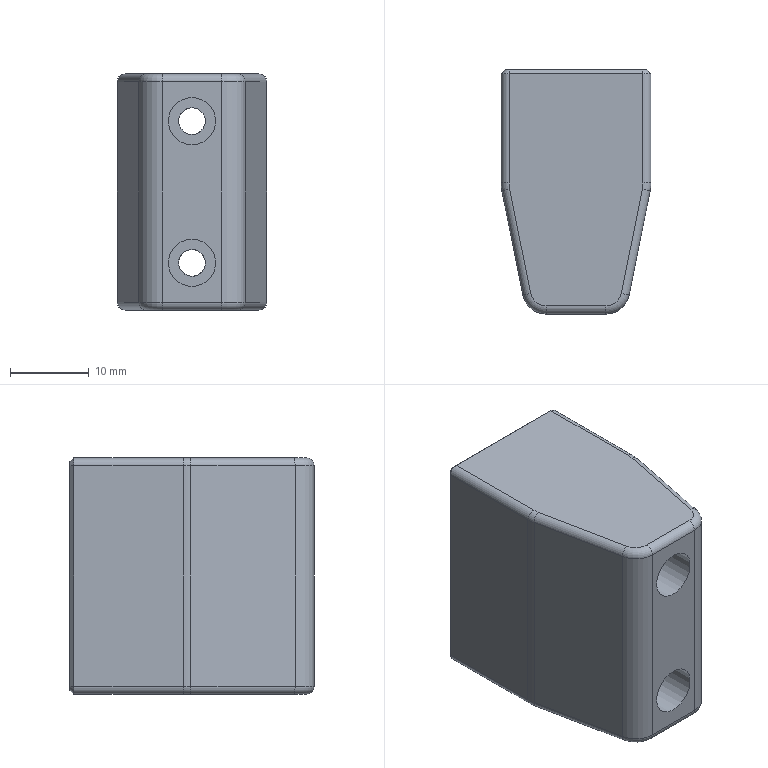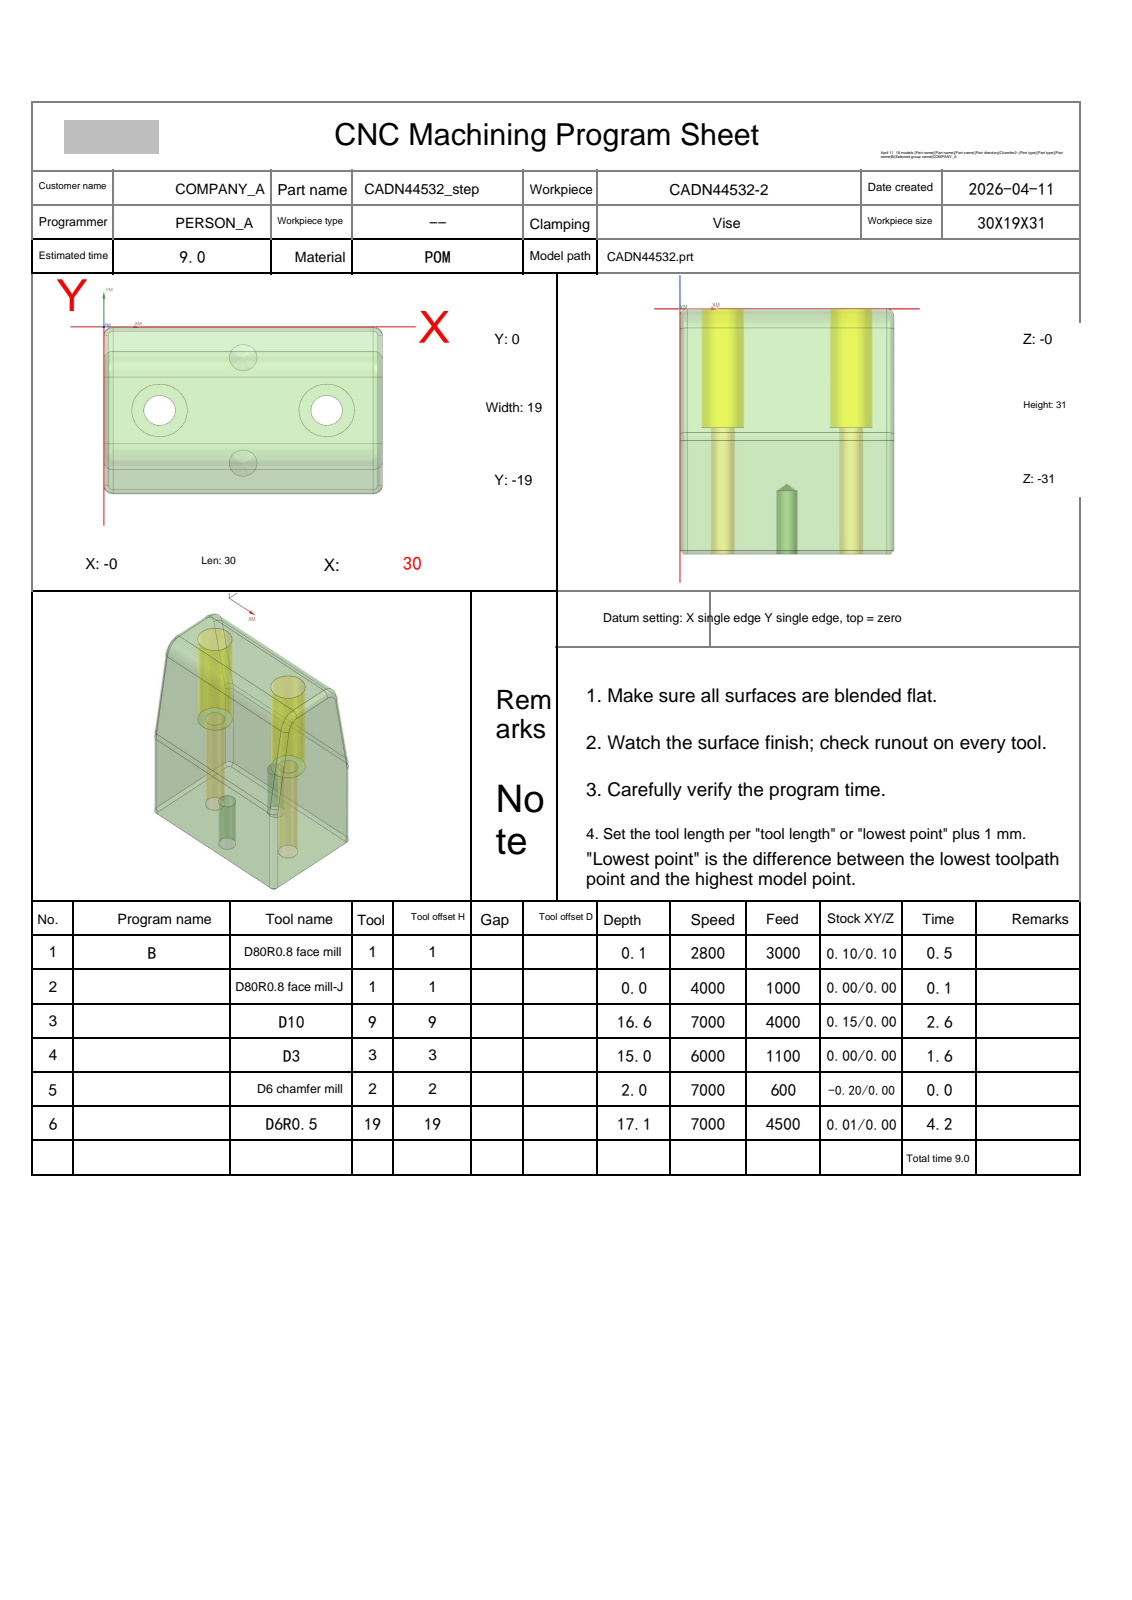NC program | NX | posted by the shop | part box 19 x 31 x 30 mm
Lines 2365 to 3536 of 6576:
N6 T19 M06
(D6R0.5  D=6. R=0.5 H=19 ce=0.01 di=0.00)
G00 G90 G54 X-2.86 Y-7.974 M03 S7000
G43 H19 Z14.8
M08
Z.492
G01 Z-.008 F4500.
G03 X-1.66 Y-6.816 I0.0 J1.2
G01 X-1.618 Y-5.615
G02 X1. Y-2.966 I2.746 J-.096
G01 X29.
G02 X31.633 Y-5.668 I-.14 J-2.77
G01 X31.66 Y-6.816
X31.702 Z-.012
X31.737 Z-.017
X31.725 Y-5.724
G03 X29. Y-2.849 I-2.912 J-.031
G01 X.999
G03 X-1.489 Y-4.634 I0.0 J-2.627
X-1.763 Y-6.296 I4.913 J-1.662
X-1.737 Y-6.816 I5.186 J0.0
G01 X-1.774 Z-.023
X-1.807 Z-.03
G02 X-1.83 Y-6.298 I5.824 J.518
X-1.667 Y-4.927 I5.847 J0.0
X1. Y-2.741 I2.779 J-.671
G01 X29.
G02 X31.795 Y-5.662 I-.16 J-2.951
G01 X31.807 Y-6.816
X31.843 Z-.037
X31.876 Z-.045
X31.863 Y-5.621
G03 X29. Y-2.635 I-3.023 J-.033
G01 X1.
G03 X-1.867 Y-5.661 I.164 J-3.027
G01 Y-5.666
X-1.865 Y-6.558
X-1.876 Y-6.816
X-1.91 Z-.054
X-1.942 Z-.063
G02 X-1.957 Y-6.31 I8.273 J.506
X-1.879 Y-5.173 I8.288 J0.0
X1. Y-2.532 I3.015 J-.397
G01 X29.
G02 X31.879 Y-5.173 I-.136 J-3.038
X31.957 Y-6.31 I-8.21 J-1.137
X31.942 Y-6.816 I-8.288 J0.0
G01 X31.975 Z-.074
X32.006 Z-.085
G03 X32.011 Y-6.458 I-13.525 J.358
X31.958 Y-5.264 I-13.53 J0.0
X29. Y-2.431 I-3.098 J-.275
G01 X1.
G03 X-1.958 Y-5.264 I.14 J-3.107
X-2.011 Y-6.458 I13.477 J-1.194
X-2.006 Y-6.816 I13.53 J0.0
G01 X-2.039 Z-.096
X-2.07 Z-.108
G02 X-2.084 Y-6.319 I8.573 J.497
X-1.982 Y-4.997 I8.587 J0.0
X1. Y-2.331 I3.117 J-.486
G01 X29.
G02 X31.982 Y-4.997 I-.135 J-3.151
X32.084 Y-6.319 I-8.485 J-1.322
X32.07 Y-6.816 I-8.587 J0.0
G01 X32.102 Z-.122
X32.132 Z-.135
G03 X32.149 Y-6.286 I-8.08 J.53
X32.017 Y-4.827 I-8.097 J0.0
X29. Y-2.233 I-3.137 J-.597
G01 X1.
G03 X-2.017 Y-4.827 I.121 J-3.191
X-2.149 Y-6.286 I7.964 J-1.459
X-2.132 Y-6.816 I8.097 J0.0
G01 X-2.163 Z-.15
X-2.193 Z-.164
G02 X-2.205 Y-6.329 I9.547 J.487
X-2.086 Y-4.827 I9.559 J0.0
X1. Y-2.136 I3.232 J-.591
G01 X29.
G02 X32.086 Y-4.827 I-.146 J-3.283
X32.205 Y-6.329 I-9.44 J-1.502
X32.193 Y-6.816 I-9.559 J0.0
G01 X32.223 Z-.18
X32.252 Z-.196
G03 X32.27 Y-6.279 I-8.146 J.538
X32.103 Y-4.637 I-8.164 J0.0
X29. Y-2.039 I-3.239 J-.716
G01 X1.
G03 X-2.103 Y-4.637 I.136 J-3.314
X-2.27 Y-6.279 I7.997 J-1.641
X-2.252 Y-6.816 I8.164 J0.0
G01 X-2.282 Z-.214
X-2.31 Z-.231
G02 X-2.316 Y-6.381 I17.318 J.436
X-2.284 Y-5.343 I17.323 J0.0
X-1.062 Y-2.75 I3.85 J-.231
X1. Y-1.945 I2.174 J-2.523
G01 X29.
G02 X31.852 Y-3.782 I-.1 J-3.287
X32.306 Y-5.736 I-3.978 J-1.954
G01 Y-6.804
X32.31 Y-6.816
X32.339 Z-.25
X32.367 Z-.269
X32.35 Y-5.519
G03 X31.934 Y-3.788 I-4.318 J-.123
X29. Y-1.851 I-3.044 J-1.419
G01 X1.
G03 X-.721 Y-2.38 I.147 J-3.539
X-2.325 Y-5.173 I2.194 J-3.117
X-2.371 Y-6.439 I17.658 J-1.266
X-2.367 Y-6.816 I17.704 J0.0
G01 X-2.395 Z-.289
X-2.422 Z-.309
G02 X-2.432 Y-6.337 I11.305 J.479
X-2.345 Y-4.938 I11.315 J0.0
X-.376 Y-2.083 I3.727 J-.464
X1. Y-1.758 I1.56 J-3.529
G01 X29.
G02 X31.758 Y-3.343 I-.091 J-3.349
G01 X31.815 Y-3.442
G02 X32.38 Y-5.173 I-3.478 J-2.092
X32.427 Y-6.39 I-15.645 J-1.217
X32.422 Y-6.816 I-15.692 J0.0
G01 X32.449 Z-.33
X32.475 Z-.351
X32.461 Y-5.519
X32.449 Y-5.319
G03 X31.678 Y-3.096 I-4.343 J-.26
X29. Y-1.667 I-2.759 J-1.946
G01 X1.
G03 X-1.02 Y-2.404 I.064 J-3.311
X-2.398 Y-4.929 I2.477 J-2.991
X-2.484 Y-6.353 I11.783 J-1.424
X-2.475 Y-6.816 I11.869 J0.0
G01 X-2.501 Z-.374
X-2.526 Z-.397
X-2.519 Y-6.558
X-2.517 Y-5.519
G02 X-1.762 Y-3.096 I4.571 J-.094
X1. Y-1.577 I2.84 J-1.893
G01 X29.
G02 X31.762 Y-3.096 I-.078 J-3.412
X32.517 Y-5.519 I-3.816 J-2.517
G01 X32.519 Y-6.804
X32.526 Y-6.816
X32.576 Z-.444
X32.57 Y-6.804
X32.566 Y-5.519
G03 X31.843 Y-3.096 I-4.627 J-.062
X29. Y-1.489 I-2.917 J-1.841
G01 X1.
G03 X-1.843 Y-3.096 I.074 J-3.448
X-2.566 Y-5.519 I3.904 J-2.485
G01 X-2.576 Y-6.816
X-2.6 Z-.47
X-2.623 Z-.495
G02 X-2.63 Y-6.334 I18.206 J.483
X-2.593 Y-5.173 I18.212 J0.0
X-1.68 Y-2.75 I4.539 J-.327
X1. Y-1.402 I2.744 J-2.117
G01 X29.
G02 X31.927 Y-3.096 I-.082 J-3.517
X32.593 Y-5.173 I-4.128 J-2.467
X32.63 Y-6.334 I-18.175 J-1.161
X32.623 Y-6.816 I-18.212 J0.0
G01 X32.646 Z-.521
X32.669 Z-.547
G03 X32.67 Y-6.517 I-28.238 J.3
X32.643 Y-5.283 I-28.24 J0.0
X31.767 Y-2.75 I-4.691 J-.205
X29. Y-1.316 I-2.846 J-2.106
G01 X1.
G03 X-1.412 Y-2.346 I.068 J-3.498
X-2.638 Y-5.173 I3.248 J-3.088
X-2.67 Y-6.517 I28.208 J-1.344
X-2.669 Y-6.816 I28.24 J0.0
G01 X-2.691 Z-.575
X-2.712 Z-.602
X-2.696 Y-5.519
G02 X-2.064 Y-3.096 I5.015 J-.014
X1. Y-1.232 I3.156 J-1.738
G01 X29.
G02 X32.064 Y-3.096 I-.092 J-3.602
X32.696 Y-5.519 I-4.384 J-2.437
G01 X32.712 Y-6.816
X32.733 Z-.631
X32.753 Z-.66
X32.754 Y-6.566
G03 X32.725 Y-5.173 I-34.209 J0.0
X32.132 Y-3.096 I-5.06 J-.322
X29. Y-1.15 I-3.218 J-1.685
G01 X1.
G03 X-.03 Y-1.317 I.355 J-5.441
X-2.307 Y-3.442 I1.237 J-3.607
X-2.739 Y-5.519 I4.983 J-2.122
G01 X-2.753 Y-6.816
X-2.772 Z-.69
X-2.791 Z-.72
G02 X-2.8 Y-6.297 I15.5 J.52
X-2.741 Y-4.942 I15.508 J0.0
X-1.991 Y-2.747 I4.83 J-.423
X1. Y-1.069 I3.072 J-1.971
G01 X29.
G02 X31.991 Y-2.747 I-.081 J-3.649
X32.741 Y-4.942 I-4.081 J-2.618
X32.8 Y-6.297 I-15.449 J-1.354
X32.791 Y-6.816 I-15.508 J0.0
G01 X32.827 Y-6.806 Z-.782
G03 X32.831 Y-6.393 I-23.233 J.414
X32.794 Y-5.093 I-23.237 J0.0
X32.06 Y-2.75 I-5.034 J-.291
X29. Y-.991 I-3.136 J-1.914
G01 X1.
G03 X-2.06 Y-2.75 I.076 J-3.673
X-2.794 Y-5.093 I4.3 J-2.635
X-2.831 Y-6.393 I23.2 J-1.299
X-2.827 Y-6.806 I23.237 J0.0
G01 X-2.86 Z-.846
X-2.855 Y-6.796
Y-5.667
G02 X-2.688 Y-4.147 I7.019 J0.0
X-1.604 Y-2.058 I4.461 J-.989
X1. Y-.914 I2.66 J-2.519
G01 X29.
G02 X31.893 Y-2.404 I-.058 J-3.665
X32.753 Y-4.481 I-3.837 J-2.806
X32.855 Y-5.764 I-8.021 J-1.283
G01 Y-5.865
Y-6.796
X32.86 Y-6.806
X32.876 Z-.879
X32.89 Z-.913
X32.888 Y-6.796
Y-5.865
Y-5.792
G03 X32.794 Y-4.515 I-8.733 J0.0
X31.964 Y-2.404 I-4.81 J-.674
X29. Y-.839 I-3.02 J-2.13
G01 X1.
G03 X-1.964 Y-2.404 I.057 J-3.695
X-2.794 Y-4.515 I3.979 J-2.785
X-2.888 Y-5.792 I8.639 J-1.277
G01 Y-5.865
Y-6.796
X-2.89 Y-6.806
X-2.904 Z-.947
X-2.917 Z-.981
X-2.912 Y-5.519
G02 X-2.676 Y-3.788 I7.099 J-.089
X-1.767 Y-2.058 I4.444 J-1.229
X1. Y-.766 I2.821 J-2.431
G01 X29.
G02 X32.103 Y-2.508 I-.059 J-3.74
X32.759 Y-4.135 I-4.133 J-2.613
X32.912 Y-5.519 I-7.222 J-1.498
G01 X32.917 Y-6.806
X32.93 Z-1.016
X32.941 Z-1.052
G03 X32.944 Y-6.385 I-34.265 J.421
X32.923 Y-5.173 I-34.268 J0.0
X32.715 Y-3.788 I-6.504 J-.269
X31.758 Y-1.964 I-4.347 J-1.117
X29. Y-.694 I-2.808 J-2.469
G01 X1.
G03 X-.03 Y-.848 I.13 J-4.412
X-2.305 Y-2.75 I1.178 J-3.721
X-2.899 Y-4.827 I4.854 J-2.512
X-2.946 Y-6.327 I24.046 J-1.5
X-2.941 Y-6.806 I24.092 J0.0
G01 X-2.952 Z-1.088
X-2.962 Z-1.124
G02 X-2.966 Y-6.335 I32.195 J.472
X-2.945 Y-5.173 I32.198 J0.0
X-2.647 Y-3.442 I6.466 J-.22
X-1.758 Y-1.881 I4.18 J-1.347
X1. Y-.625 I2.814 J-2.524
G01 X29.
G02 X32.103 Y-2.322 I-.064 J-3.803
X32.749 Y-3.788 I-3.957 J-2.619
X32.945 Y-5.173 I-6.558 J-1.632
X32.966 Y-6.335 I-32.177 J-1.162
X32.962 Y-6.806 I-32.198 J0.0
G01 X32.971 Z-1.162
X32.979 Z-1.199
G03 X32.985 Y-6.272 I-24.736 J.534
X32.943 Y-4.827 I-24.741 J0.0
X32.681 Y-3.442 I-5.484 J-.321
G01 X32.565 Y-3.096
G03 X31.669 Y-1.712 I-3.959 J-1.578
X29. Y-.558 I-2.714 J-2.616
G01 X1.
G03 X-.768 Y-1.019 I.061 J-3.857
X-2.623 Y-3.269 I2.012 J-3.548
G01 X-2.681 Y-3.442
G03 X-2.943 Y-4.827 I5.407 J-1.741
X-2.985 Y-6.272 I24.699 J-1.446
X-2.979 Y-6.806 I24.741 J0.0
G01 X-2.993 Z-1.275
X-2.989 Y-6.796
X-2.988 Y-5.519
Y-5.491
G02 X-2.884 Y-4.135 I8.893 J0.0
X-2.715 Y-3.442 I3.626 J-.516
X-.721 Y-.927 I3.944 J-1.079
X1. Y-.494 I1.78 J-3.433
G01 X29.
G02 X31.758 Y-1.728 I-.045 J-3.8
G01 X31.946 Y-1.955
G02 X32.715 Y-3.442 I-3.055 J-2.523
X32.871 Y-4.065 I-3.863 J-1.295
X32.988 Y-5.478 I-8.443 J-1.413
G01 Y-5.519
X32.989 Y-6.796
X32.993 Y-6.806
X33.003 Z-1.353
X32.991 Y-5.173
G03 X32.905 Y-4.135 I-6.688 J-.028
G01 X32.846 Y-3.788
G03 X32.449 Y-2.65 I-5.214 J-1.179
G01 X32.312 Y-2.404
G03 X29. Y-.431 I-3.37 J-1.891
G01 X1.
G03 X-1.412 Y-1.323 I.049 J-3.841
X-2.641 Y-3.096 I2.753 J-3.221
X-2.981 Y-4.827 I5.714 J-2.02
G01 X-2.991 Y-5.173
X-3.003 Y-6.806
X-3.009 Z-1.433
X-2.999 Y-5.173
G02 X-2.865 Y-3.788 I7.288 J-.005
X-2.357 Y-2.404 I4.303 J-.793
G01 X-2.148 Y-2.058
G02 X1. Y-.371 I3.204 J-2.198
G01 X29.
G02 X32.148 Y-2.058 I-.056 J-3.884
G01 X32.357 Y-2.404
G02 X32.867 Y-3.788 I-3.868 J-2.21
X32.989 Y-4.827 I-6.47 J-1.285
X33.011 Y-6.334 I-51.964 J-1.507
X33.009 Y-6.806 I-51.986 J0.0
G01 Y-6.801 Z-1.515
G03 X33.013 Y-6.198 I-47.709 J.603
X32.987 Y-4.615 I-47.713 J0.0
X32.409 Y-2.414 I-5.127 J-.17
X29. Y-.313 I-3.465 J-1.806
G01 X1.
G03 X-1.609 Y-1.365 I.048 J-3.878
X-2.707 Y-3.096 I2.888 J-3.045
X-2.982 Y-4.481 I5.418 J-1.796
G01 X-2.996 Y-4.827
X-3.007 Y-5.173
X-3.009 Y-6.801
X-3.01 Z-1.598
X-3.009 Y-5.173
X-3.004 Y-4.827
G02 X-2.833 Y-3.442 I5.809 J-.012
G01 X-2.794 Y-3.267
X-2.696 Y-2.98
G02 X-.721 Y-.675 I3.884 J-1.329
X1. Y-.257 I1.798 J-3.657
G01 X29.
G02 X30.721 Y-.675 I-.077 J-4.074
X32.45 Y-2.404 I-1.933 J-3.662
X32.973 Y-4.262 I-4.467 J-2.26
X33.009 Y-5.166 I-11.232 J-.903
G01 Y-5.173
Y-6.801
Z-1.683
Y-4.827
G03 X32.926 Y-3.788 I-6.967 J-.033
X32.285 Y-2.058 I-4.445 J-.662
X29.946 Y-.327 I-3.365 J-2.102
X29. Y-.204 I-1.184 J-5.417
G01 X1.
G03 X.054 Y-.327 I.239 J-5.54
X-2.485 Y-2.404 I1.048 J-3.872
X-2.996 Y-4.481 I4.493 J-2.205
G01 X-3.009 Y-4.827
X-3.01 Y-6.801
Z-1.769
G02 X-3.02 Y-5.855 I44.13 J.946
X-2.992 Y-4.283 I44.14 J0.0
X-2.33 Y-2.06 I4.615 J-.164
X1. Y-.153 I3.38 J-2.041
G01 X29.
G02 X30.721 Y-.57 I-.063 J-4.021
X32.521 Y-2.404 I-1.834 J-3.601
X33.003 Y-4.481 I-4.485 J-2.134
G01 X33.009 Y-4.827
Y-6.801
X33.01 Z-1.857
X33.009 Y-4.481
G03 X32.812 Y-3.089 I-5.442 J-.061
X32.222 Y-1.839 I-3.931 J-1.089
G01 X32.103 Y-1.669
G03 X29. Y-.105 I-3.147 J-2.385
G01 X1.
G03 X-2.552 Y-2.404 I.055 J-3.978
X-3.009 Y-4.481 I4.5 J-2.079
G01 X-3.01 Y-6.801
Z-1.946
X-3.009 Y-4.481
X-3.01 Y-4.419
G02 X-2.723 Y-2.75 I5.008 J0.0
X-1.077 Y-.673 I3.861 J-1.369
X1. Y-.059 I2.12 J-3.352
G01 X29.
G02 X31.898 Y-1.365 I-.038 J-3.953
X32.912 Y-3.442 I-3.193 J-2.846
X33.009 Y-4.478 I-5.483 J-1.036
G01 Y-4.481
X33.01 Y-6.801
Z-2.036
X33.009 Y-4.347
G03 X32.85 Y-3.09 I-5.049 J-.001
X32.103 Y-1.56 I-4.101 J-1.055
X30.721 Y-.428 I-3.094 J-2.368
X29. Y-.016 I-1.775 J-3.617
G01 X1.
G03 X-1.758 Y-1.168 I.04 J-3.974
X-2.607 Y-2.404 I2.88 J-2.889
G01 X-2.745 Y-2.75
G03 X-3.002 Y-4.135 I4.316 J-1.518
G01 X-3.009 Y-4.481
X-3.01 Y-6.801
Z-2.128
X-3.009 Y-4.481
X-3.007 Y-4.135
G02 X-2.632 Y-2.404 I4.58 J-.087
X-.03 Y-.12 I3.686 J-1.574
X1. Y.024 I1.164 J-4.575
G01 X29.
G02 X30.03 Y-.12 I-.134 J-4.718
X32.632 Y-2.404 I-1.084 J-3.859
X33.007 Y-4.135 I-4.188 J-1.813
G01 X33.009 Y-4.481
X33.01 Y-6.801
Z-2.22
X33.009 Y-4.113
G03 X32.596 Y-2.283 I-4.268 J-.001
G01 X32.555 Y-2.196
G03 X29.586 Y.011 I-3.563 J-1.692
X29. Y.062 I-.693 J-4.559
G01 X1.
G03 X-.03 Y-.079 I.108 J-4.61
X-2.449 Y-1.98 I1.081 J-3.864
X-3.009 Y-4.135 I3.924 J-2.171
G01 X-3.01 Y-6.801
Z-2.314
X-3.009 Y-4.135
X-3.01 Y-4.085
G02 X-2.514 Y-2.058 I4.394 J0.0
X.315 Y.034 I3.541 J-1.829
X1. Y.097 I1.065 J-7.807
G01 X29.
G02 X31.335 Y-.673 I-.056 J-4.091
X33.01 Y-4.049 I-2.563 J-3.376
G01 X33.009 Y-4.135
X33.01 Y-6.801
Z-2.409
X33.009 Y-4.135
X33.01 Y-4.048
G03 X32.698 Y-2.404 I-4.483 J0.0
X29. Y.13 I-3.73 J-1.479
G01 X1.
G03 X-1.379 Y-.673 I.034 J-4.028
X-2.998 Y-3.788 I2.512 J-3.284
G01 X-3.009 Y-4.135
X-3.01 Y-6.801
Z-2.504
X-3.009 Y-4.135
X-3.002 Y-3.788
G02 X-1.814 Y-1.019 I4.149 J-.141
X.315 Y.099 I2.847 J-2.836
X1. Y.16 I1.256 J-10.176
G01 X29.
G02 X29.685 Y.099 I-.572 J-10.237
G01 X30.03 Y.02
X30.376 Y-.093
X30.721 Y-.238
G02 X32.794 Y-2.624 I-1.812 J-3.668
G01 X32.864 Y-2.88
G02 X33.009 Y-3.955 I-3.922 J-1.076
G01 X33.01 Y-6.801
Z-2.6
X33.009 Y-3.893
G03 X32.695 Y-2.33 I-4.051 J-.001
X32.449 Y-1.815 I-5.271 J-2.207
X30.376 Y-.063 I-3.495 J-2.033
X29. Y.187 I-1.46 J-4.123
G01 X1.
G03 X.558 Y.152 I.484 J-8.954
X-1.412 Y-.639 I.399 J-3.843
X-2.57 Y-2.058 I2.323 J-3.077
X-3.005 Y-3.788 I3.567 J-1.818
G01 X-3.009 Y-4.135
X-3.01 Y-6.801
Z-2.697
X-3.009 Y-3.788
G02 X-1.87 Y-1.019 I4.134 J-.081
X1. Y.211 I2.903 J-2.809
G01 X29.
G02 X32.449 Y-1.784 I-.032 J-4.034
X33.009 Y-3.788 I-3.72 J-2.12
G01 X33.01 Y-6.801
Z-2.795
X33.009 Y-3.788
G03 X30.721 Y-.161 I-4.075 J-.036
X29. Y.233 I-1.766 J-3.759
G01 X1.
G03 X-.721 Y-.161 I.045 J-4.153
X-3.009 Y-3.788 I1.786 J-3.662
G01 X-3.01 Y-6.801
Z-2.892
X-3.009 Y-3.788
G02 X-.03 Y.117 I4.05 J-.001
X1. Y.252 I1.109 J-4.446
G01 X29.
G02 X31.067 Y-.326 I-.038 J-4.12
X33.009 Y-3.788 I-2.136 J-3.475
G01 X33.01 Y-6.801
Z-2.99
X33.009 Y-3.788
Y-3.778
G03 X31.758 Y-.836 I-4.084 J0.0
X29. Y.272 I-2.787 J-2.951
G01 X1.
G03 X-.03 Y.136 I.074 J-4.542
X-3.009 Y-3.766 I1.066 J-3.902
G01 Y-3.788
X-3.01 Y-6.801
Z-3.088
X-3.009 Y-3.788
X-3.01 Y-3.74
G02 X1. Y.292 I4.032 J0.0
G01 X29.
G02 X31.954 Y-1.019 I-.022 J-4.034
X33.009 Y-3.755 I-3.017 J-2.736
G01 Y-3.788
X33.01 Y-6.801
Z-3.185
X33.009 Y-3.788
X33.01 Y-3.727
G03 X32.833 Y-2.555 I-3.975 J0.0
X29. Y.311 I-3.849 J-1.151
G01 X1.
G03 X-3.01 Y-3.72 I.022 J-4.032
G01 X-3.009 Y-3.788
X-3.01 Y-6.801
Z-3.283
X-3.009 Y-3.788
X-3.01 Y-3.701
G02 X1. Y.331 I4.032 J0.0
G01 X29.
G02 X32.834 Y-2.534 I-.013 J-4.015
X33.01 Y-3.713 I-3.851 J-1.179
G01 X33.009 Y-3.788
X33.01 Y-6.801
Z-3.381
X33.009 Y-3.675
G03 X32.594 Y-1.914 I-3.94 J-.001
G01 X32.492 Y-1.712
G03 X29. Y.351 I-3.5 J-1.939
G01 X1.
G03 X-3. Y-3.442 I.017 J-4.024
G01 X-3.009 Y-3.788
X-3.01 Y-6.801
Z-3.479
X-3.009 Y-3.788
X-3.001 Y-3.442
G02 X1. Y.371 I4.019 J-.211
G01 X29.
G02 X32.673 Y-2.054 I-.011 J-4.011
X33.009 Y-3.686 I-3.791 J-1.633
G01 X33.01 Y-6.801
Z-3.577
X33.009 Y-3.631
G03 X32.858 Y-2.57 I-3.808 J-.001
G01 X32.794 Y-2.349
G03 X29. Y.39 I-3.808 J-1.277
G01 X1.
G03 X-3.002 Y-3.442 I.018 J-4.025
G01 X-3.009 Y-3.788
X-3.01 Y-6.801
Z-3.675
X-3.009 Y-3.788
X-3.003 Y-3.442
G02 X1. Y.41 I4.022 J-.173
G01 X29.
G02 X32.84 Y-2.49 I-.009 J-4.005
X33.009 Y-3.593 I-3.517 J-1.104
G01 X33.01 Y-6.801
Z-3.773
X33.009 Y-3.577
G03 X32.846 Y-2.49 I-3.701 J-.001
X29. Y.43 I-3.855 J-1.085
G01 X1.
G03 X-3.004 Y-3.442 I.018 J-4.026
G01 X-3.009 Y-3.788
X-3.01 Y-6.801
Z-3.871
X-3.009 Y-3.788
X-3.005 Y-3.442
G02 X1. Y.45 I4.024 J-.134
G01 X29.
G02 X32.827 Y-2.404 I-.01 J-4.007
G01 X32.867 Y-2.544
G02 X33.009 Y-3.568 I-3.621 J-1.025
G01 X33.01 Y-6.801
Z-3.969
X33.009 Y-3.788
X33.007 Y-3.442
G03 X32.858 Y-2.49 I-3.675 J-.087
X29. Y.47 I-3.868 J-1.047
G01 X1.
G03 X-3.006 Y-3.442 I.02 J-4.028
G01 X-3.009 Y-3.788
X-3.01 Y-6.801
Z-4.067
X-3.009 Y-3.788
X-3.008 Y-3.442
G02 X1. Y.489 I4.028 J-.097
G01 X29.
G02 X32.864 Y-2.49 I-.011 J-4.008
X33.008 Y-3.442 I-3.665 J-1.042
G01 X33.009 Y-3.788
X33.01 Y-6.801
Z-4.165
X33.009 Y-3.788
Y-3.53
G03 X32.152 Y-1.035 I-4.089 J-.01
X29. Y.509 I-3.151 J-2.443
G01 X1.
G03 X-3.009 Y-3.442 I.021 J-4.03
G01 Y-3.788
X-3.01 Y-6.801
Z-4.263
X-3.009 Y-3.442
G02 X1. Y.529 I4.03 J-.059
G01 X29.
G02 X33.009 Y-3.442 I-.022 J-4.031
G01 X33.01 Y-6.801
Z-4.361
X33.009 Y-3.442
G03 X29. Y.549 I-4.03 J-.039
G01 X1.
G03 X-3.009 Y-3.442 I.021 J-4.03
G01 X-3.01 Y-6.801
Z-4.459
X-3.009 Y-3.442
G02 X1. Y.568 I4.03 J-.019
G01 X29.
G02 X33.009 Y-3.442 I-.021 J-4.03
G01 X33.01 Y-6.801
Z-4.557
X33.009 Y-3.442
G03 X29. Y.588 I-4.03 J0.0
G01 X1.
G03 X-3.009 Y-3.441 I.02 J-4.03
G01 X-3.01 Y-6.801
Z-4.656
X-3.009 Y-3.442
Y-3.421
G02 X1. Y.608 I4.029 J0.0
G01 X29.
G02 X33.009 Y-3.421 I-.02 J-4.029
G01 Y-3.442
X33.01 Y-6.801
Z-4.754
X33.009 Y-3.442
X33.01 Y-3.402
G03 X29. Y.628 I-4.03 J0.0
G01 X1.
G03 X-3.01 Y-3.402 I.02 J-4.029
G01 X-3.009 Y-3.442
X-3.01 Y-6.801
Z-4.852
X-3.009 Y-3.442
X-3.01 Y-3.382
G02 X1. Y.647 I4.03 J0.0
G01 X29.
G02 X32.994 Y-3.096 I-.014 J-4.018
G01 X33.009 Y-3.442
X33.01 Y-6.801
Z-4.95
X33.009 Y-3.442
X32.996 Y-3.096
G03 X29. Y.667 I-4.01 J-.254
G01 X1.
G03 X-3.01 Y-3.363 I.02 J-4.03
G01 X-3.009 Y-3.442
X-3.01 Y-6.801
Z-5.048
X-3.009 Y-3.442
X-2.998 Y-3.096
G02 X1. Y.687 I4.013 J-.237
G01 X29.
G02 X32.997 Y-3.096 I-.014 J-4.018
G01 X33.009 Y-3.442
X33.01 Y-6.801
Z-5.146
X33.009 Y-3.442
X32.998 Y-3.096
G03 X29. Y.707 I-4.013 J-.216
G01 X1.
G03 X-2.999 Y-3.096 I.016 J-4.021
G01 X-3.009 Y-3.442
X-3.01 Y-6.801
Z-5.244
X-3.009 Y-3.442
X-3.001 Y-3.096
G02 X1. Y.726 I4.017 J-.199
G01 X29.
G02 X33. Y-3.096 I-.016 J-4.02
G01 X33.009 Y-3.442
X33.01 Y-5.173
Y-6.801
Z-5.342
X33.009 Y-3.442
X33.001 Y-3.096
G03 X29. Y.746 I-4.017 J-.179
G01 X1.
G03 X-3.002 Y-3.096 I.017 J-4.023
G01 X-3.009 Y-3.442
X-3.01 Y-6.801
Z-5.44
X-3.009 Y-3.442
X-3.003 Y-3.096
G02 X1. Y.766 I4.021 J-.162
G01 X29.
G02 X33.002 Y-3.096 I-.017 J-4.022
G01 X33.009 Y-3.442
X33.01 Y-6.801
Z-5.538
X33.009 Y-3.442
X33.004 Y-3.096
G03 X29. Y.786 I-4.021 J-.142
G01 X1.
G03 X-3.004 Y-3.096 I.018 J-4.025
G01 X-3.009 Y-3.442
X-3.01 Y-6.801
Z-5.636
X-3.009 Y-3.442
X-3.005 Y-3.096
G02 X1. Y.806 I4.026 J-.126
G01 X29.
G02 X33.005 Y-3.096 I-.018 J-4.025
G01 X33.009 Y-3.442
X33.01 Y-6.801
Z-5.734
X33.009 Y-3.442
X33.006 Y-3.096
G03 X29. Y.825 I-4.026 J-.106
G01 X1.
G03 X-.03 Y.69 I.049 J-4.352
X-3.007 Y-3.096 I1.064 J-3.9
G01 X-3.009 Y-3.442
X-3.01 Y-6.801
Z-5.832
X-3.009 Y-3.442
X-3.008 Y-3.096
G02 X-.721 Y.452 I4.052 J-.1
X.992 Y.845 I1.713 J-3.542
G01 X29.
G02 X33.008 Y-3.096 I-.02 J-4.029
G01 X33.009 Y-3.442
X33.01 Y-6.801
Z-5.93
X33.009 Y-3.096
G03 X29. Y.865 I-4.03 J-.069
G01 X1.
G03 X-.721 Y.472 I.012 J-4.02
X-3.009 Y-3.096 I1.766 J-3.65
G01 X-3.01 Y-6.801
Z-6.028
X-3.009 Y-3.096
G02 X-.03 Y.749 I4.045 J-.058
X1. Y.885 I1.076 J-4.194
G01 X29.
G02 X33.009 Y-3.096 I-.021 J-4.03
G01 X33.01 Y-6.558
Y-6.801
Z-6.126
X33.009 Y-3.096
G03 X29. Y.904 I-4.03 J-.03
G01 X1.
G03 X-.03 Y.769 I.046 J-4.329
X-3.009 Y-3.096 I1.065 J-3.901
G01 X-3.01 Y-6.801
Z-6.224
X-3.009 Y-3.096
G02 X1. Y.924 I4.032 J-.012
G01 X29.
G02 X33.009 Y-3.096 I-.021 J-4.03
G01 X33.01 Y-6.801
Z-6.322
X33.009 Y-3.096
Y-3.086
G03 X29. Y.944 I-4.03 J0.0
G01 X1.
G03 X-3.009 Y-3.086 I.02 J-4.03
G01 Y-3.096
X-3.01 Y-6.801
Z-6.42
X-3.009 Y-3.096
Y-3.066
G02 X1. Y.964 I4.029 J0.0
G01 X29.
G02 X33.009 Y-3.065 I-.019 J-4.029
G01 Y-3.096
X33.01 Y-6.801
Z-6.518
X33.009 Y-3.096
X33.01 Y-3.048
G03 X29. Y.983 I-4.032 J0.0
G01 X1.
G03 X-3.01 Y-3.046 I.02 J-4.03
G01 X-3.009 Y-3.096
X-3.01 Y-6.801
Z-6.616
X-3.009 Y-3.096
X-3.01 Y-3.027
G02 X1. Y1.003 I4.03 J0.0
G01 X29.
G02 X32.995 Y-2.75 I-.014 J-4.018
G01 X33.009 Y-3.096
X33.01 Y-6.801
Z-6.714
X33.009 Y-3.096
X32.996 Y-2.75
G03 X29. Y1.023 I-4.01 J-.245
G01 X1.
G03 X-3.01 Y-3.008 I.02 J-4.031
G01 X-3.009 Y-3.096
X-3.01 Y-6.801
Z-6.812
X-3.009 Y-3.096
X-2.999 Y-2.75
G02 X1. Y1.043 I4.014 J-.228
G01 X29.
G02 X32.998 Y-2.75 I-.014 J-4.018
G01 X33.009 Y-3.096
X33.01 Y-6.801
Z-6.91
Y-4.827
X33.009 Y-3.096
X32.999 Y-2.75
G03 X29. Y1.062 I-4.014 J-.206
G01 X1.
G03 X-3. Y-2.75 I.016 J-4.021
G01 X-3.009 Y-3.096
X-3.01 Y-6.801
Z-7.008
X-3.009 Y-3.096
X-3.001 Y-2.75
G02 X1. Y1.082 I4.018 J-.19
G01 X29.
G02 X33. Y-2.75 I-.016 J-4.02
G01 X33.009 Y-3.096
X33.01 Y-4.827
Y-6.801
Z-7.106
X33.009 Y-3.096
X33.002 Y-2.75
G03 X29. Y1.102 I-4.018 J-.17
G01 X1.
G03 X-3.002 Y-2.75 I.018 J-4.024
G01 X-3.009 Y-3.096
X-3.01 Y-6.801
Z-7.204
X-3.009 Y-3.096
X-3.004 Y-2.75
G02 X1. Y1.122 I4.022 J-.153
G01 X29.
G02 X33.003 Y-2.75 I-.017 J-4.023
G01 X33.009 Y-3.096
X33.01 Y-6.801
Z-7.302
X33.009 Y-3.096
X33.004 Y-2.75
G03 X29. Y1.141 I-4.023 J-.133
G01 X1.
G03 X-3.005 Y-2.75 I.019 J-4.026
G01 X-3.009 Y-3.096
X-3.01 Y-6.801
Z-7.4
X-3.009 Y-3.096
X-3.006 Y-2.75
G02 X1. Y1.161 I4.028 J-.119
G01 X29.
G02 X33.006 Y-2.75 I-.021 J-4.028
G01 X33.009 Y-3.096
X33.01 Y-6.801
Z-7.498
X33.009 Y-3.096
X33.007 Y-2.75
G03 X32.839 Y-1.712 I-3.851 J-.092
X29. Y1.181 I-3.849 J-1.114
G01 X1.
G03 X-.03 Y1.045 I.048 J-4.343
X-3.007 Y-2.75 I1.065 J-3.901
G01 X-3.009 Y-3.096
X-3.01 Y-6.801
Z-7.596
X-3.009 Y-3.096
Y-2.75
G02 X-.721 Y.808 I4.054 J-.092
X1. Y1.201 I1.732 J-3.624
G01 X29.
G02 X32.931 Y-2.058 I-.015 J-4.019
X33.008 Y-2.75 I-3.919 J-.788
G01 X33.009 Y-3.096
X33.01 Y-6.801
Z-7.694
X33.009 Y-2.75
X32.995 Y-2.534
G03 X29. Y1.221 I-4.011 J-.265
G01 X.992
G03 X-.721 Y.828 I0.0 J-3.933
X-3.009 Y-2.75 I1.766 J-3.65
G01 X-3.01 Y-6.801
Z-7.792
X-3.009 Y-2.75
G02 X-.03 Y1.105 I4.045 J-.047
X1. Y1.24 I1.076 J-4.194
G01 X29.
G02 X32.998 Y-2.555 I-.016 J-4.02
G01 X33.009 Y-2.75
X33.01 Y-6.558
Y-6.801
Z-7.89
X33.009 Y-2.75
X32.999 Y-2.555
G03 X29. Y1.26 I-4.015 J-.205
G01 X1.
G03 X-.03 Y1.124 I.046 J-4.329
X-3.009 Y-2.75 I1.064 J-3.901
G01 X-3.01 Y-6.801
Z-7.988
X-3.009 Y-2.75
G02 X1. Y1.28 I4.031 J-.001
G01 X29.
G02 X33.009 Y-2.75 I-.023 J-4.032
G01 X33.01 Y-6.801
Z-8.086
X33.009 Y-2.75
Y-2.731
G03 X29. Y1.3 I-4.031 J0.0
G01 X1.
G03 X-3.003 Y-2.555 I.016 J-4.022
G01 X-3.009 Y-2.75
X-3.01 Y-6.801
Z-8.185
X-3.009 Y-2.75
X-3.004 Y-2.555
G02 X1. Y1.319 I4.02 J-.148
G01 X29.
G02 X33.01 Y-2.71 I-.02 J-4.03
G01 X33.009 Y-2.75
X33.01 Y-6.801
Z-8.283
X33.009 Y-2.75
X33.005 Y-2.555
G03 X29. Y1.339 I-4.022 J-.129
G01 X1.
G03 X-3.005 Y-2.555 I.017 J-4.024
G01 X-3.009 Y-2.75
X-3.01 Y-6.801
Z-8.381
X-3.009 Y-2.75
X-3.006 Y-2.555
G02 X1. Y1.359 I4.024 J-.112
G01 X29.
G02 X33.006 Y-2.555 I-.018 J-4.025
G01 X33.009 Y-2.75
X33.01 Y-6.801
Z-8.479
X33.009 Y-2.75
X33.007 Y-2.555
G03 X29. Y1.379 I-4.026 J-.093
G01 X1.
G03 X-3.007 Y-2.555 I.019 J-4.027
G01 X-3.009 Y-2.75
X-3.01 Y-6.801
Z-8.577
X-3.009 Y-2.75
Y-2.555
G02 X1. Y1.398 I4.029 J-.076
G01 X29.
G02 X33.009 Y-2.555 I-.019 J-4.029
G01 Y-2.75
X33.01 Y-6.801
Z-8.675
X33.009 Y-2.534
G03 X29. Y1.418 I-4.028 J-.077
G01 X1.
G03 X-3.009 Y-2.534 I.021 J-4.031
G01 Y-2.75
X-3.01 Y-6.801
Z-8.773
X-3.009 Y-2.534
X-3.007 Y-2.49
G02 X1. Y1.438 I4.027 J-.1
G01 X29.
G02 X33.007 Y-2.49 I-.019 J-4.027
G01 X33.009 Y-2.534
X33.01 Y-6.801
Z-8.871
X33.008 Y-2.49
G03 X29. Y1.458 I-4.031 J-.083
G01 X.993
G03 X-.721 Y1.065 I0.0 J-3.937
X-3.009 Y-2.555 I1.764 J-3.648
G01 X-3.01 Y-6.801
Z-8.969
X-3.009 Y-2.49
X-3.004 Y-2.404
G02 X1. Y1.477 I4.022 J-.144
G01 X29.
G02 X32.978 Y-2.058 I-.021 J-4.029
G01 X32.982 Y-2.09
X33.004 Y-2.404
X33.009 Y-2.49
X33.01 Y-6.801
Z-9.067
X33.009 Y-2.49
X33.005 Y-2.404
G03 X29. Y1.497 I-4.024 J-.125
G01 X1.
G03 X-3.005 Y-2.404 I.02 J-4.028
G01 X-3.009 Y-2.49
X-3.01 Y-6.801
Z-9.165
X-3.009 Y-2.523
G02 X-.721 Y1.124 I4.053 J-.001
X.992 Y1.517 I1.713 J-3.542
G01 X29.
G02 X32.836 Y-1.365 I-.01 J-4.007
X33.009 Y-2.517 I-3.731 J-1.152
G01 Y-2.55
X33.01 Y-6.801
Z-9.263
X33.009 Y-2.55
Y-2.503
Y-2.502
G03 X32.842 Y-1.365 I-3.933 J0.0
X29. Y1.537 I-3.851 J-1.104
G01 X.992
G03 X-.721 Y1.144 I0.0 J-3.934
X-3.009 Y-2.503 I1.765 J-3.649
G01 Y-2.55
X-3.01 Y-6.801
Z-9.361
X-3.009 Y-2.55
Y-2.484
G02 X-.721 Y1.164 I4.054 J-.001
X.992 Y1.557 I1.713 J-3.541
G01 X29.
G02 X32.847 Y-1.365 I-.01 J-4.007
X33.009 Y-2.484 I-3.876 J-1.133
G01 Y-2.55
X33.01 Y-6.801
Z-9.459
X33.009 Y-2.55
Y-2.464
G03 X32.853 Y-1.365 I-4.063 J-.017
G01 X32.794 Y-1.163
G03 X29. Y1.576 I-3.808 J-1.277
G01 X1.
G03 X-.03 Y1.441 I.046 J-4.329
X-3.009 Y-2.461 I1.066 J-3.902
G01 Y-2.464
Y-2.55
X-3.01 Y-6.801
Z-9.557
X-3.009 Y-2.55
Y-2.444
Y-2.441
G02 X-.03 Y1.46 I4.044 J0.0
X1. Y1.596 I1.076 J-4.194
G01 X29.
G02 X32.794 Y-1.143 I-.013 J-4.016
G01 X32.859 Y-1.365
G02 X33.009 Y-2.444 I-3.934 J-1.099
G01 Y-2.55
X33.01 Y-6.801
Z-9.655
X33.009 Y-2.55
Y-2.424
G03 X32.864 Y-1.365 I-4.106 J-.022
G01 X32.794 Y-1.123
G03 X29. Y1.616 I-3.807 J-1.276
G01 X1.
G03 X-3.009 Y-2.417 I.023 J-4.033
G01 Y-2.424
Y-2.55
X-3.01 Y-6.801
Z-9.753
X-3.009 Y-2.55
Y-2.405
Y-2.394
G02 X1. Y1.636 I4.03 J0.0
G01 X29.
G02 X33.009 Y-2.396 I-.022 J-4.032
G01 Y-2.405
Y-2.55
X33.01 Y-6.801
Z-9.851
X33.009 Y-2.55
Y-2.385
Y-2.373
G03 X29. Y1.655 I-4.028 J0.0
G01 X1.
G03 X-3.009 Y-2.376 I.023 J-4.032
G01 Y-2.385
Y-2.55
X-3.01 Y-6.801
Z-9.949
X-3.009 Y-2.55
Y-2.365
Y-2.352
G02 X1. Y1.675 I4.027 J0.0
G01 X29.
G02 X33.008 Y-2.353 I-.019 J-4.028
G01 Y-2.365
X33.009 Y-2.55
X33.01 Y-6.801
Z-10.047
X33.009 Y-2.55
X33.008 Y-2.345
Y-2.333
G03 X29. Y1.695 I-4.028 J0.0
G01 X1.
G03 X-3.009 Y-2.333 I.019 J-4.028
G01 Y-2.345
Y-2.55
X-3.01 Y-6.801
Z-10.145
X-3.009 Y-2.55
Y-2.326
Y-2.315
G02 X1. Y1.715 I4.03 J0.0
G01 X29.
G02 X33.009 Y-2.316 I-.021 J-4.03
G01 Y-2.326
Y-2.55
X33.01 Y-6.801
Z-10.243
X33.009 Y-2.55
Y-2.306
Y-2.293
G03 X29. Y1.734 I-4.028 J0.0
G01 X1.
G03 X-3.009 Y-2.293 I.018 J-4.028
G01 Y-2.306
Y-2.55
X-3.01 Y-6.801
Z-10.341
X-3.009 Y-2.55
Y-2.286
Y-2.275
G02 X1. Y1.754 I4.029 J0.0
G01 X29.
G02 X33.009 Y-2.275 I-.02 J-4.029
G01 Y-2.286
Y-2.55
X33.01 Y-6.801
Z-10.439
X33.009 Y-2.55
Y-2.266